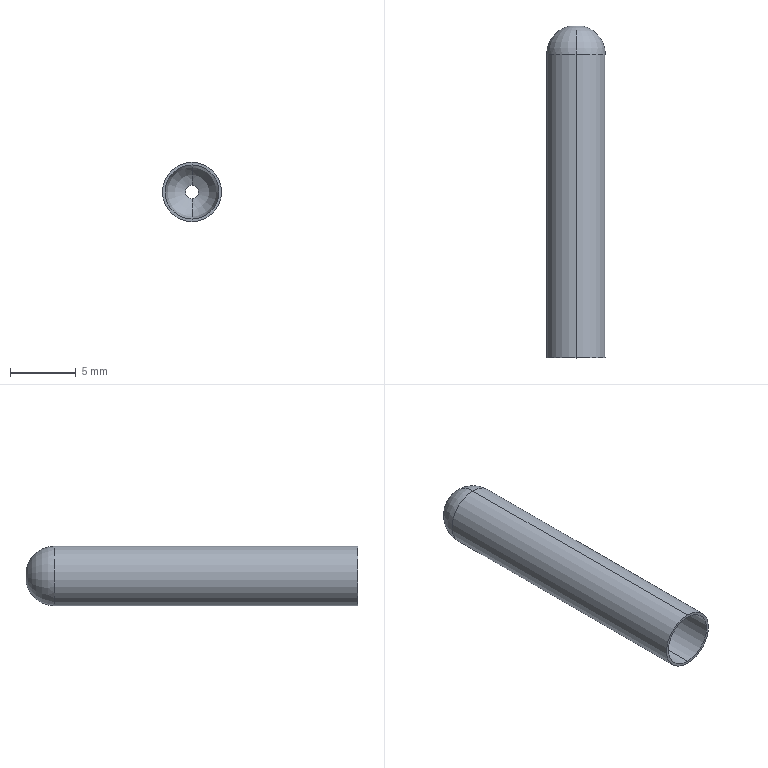Part | SolidWorks | features Revolution 1 | 1 solid | 11 faces | box 4.5 x 25.2 x 4.5 mm | volume 67.862 mm3 | cylinder 6 | torus 4 | plane 1 | commonest cylinder face diameters 1 x2 4.1 x2 4.5 x2
STEP:
#1=CARTESIAN_POINT('',(0.,23.047,2.05));
#2=VERTEX_POINT('',#1);
#3=CARTESIAN_POINT('',(0.,23.047,-2.05));
#4=VERTEX_POINT('',#3);
#5=CARTESIAN_POINT('',(0.,23.047,0.));
#6=DIRECTION('',(0.,-1.,0.));
#7=DIRECTION('',(0.,0.,-1.));
#8=AXIS2_PLACEMENT_3D('',#5,#6,#7);
#9=CIRCLE('',#8,2.05);
#10=EDGE_CURVE('',#2,#4,#9,.T.);
#11=ORIENTED_EDGE('',*,*,#10,.F.);
#12=CARTESIAN_POINT('',(0.,0.,2.05));
#13=VERTEX_POINT('',#12);
#14=CARTESIAN_POINT('',(0.,0.,2.05));
#15=DIRECTION('',(0.,-1.,0.));
#16=VECTOR('',#15,1000.);
#17=LINE('',#14,#16);
#18=EDGE_CURVE('',#2,#13,#17,.T.);
#19=ORIENTED_EDGE('',*,*,#18,.T.);
#20=CARTESIAN_POINT('',(0.,0.,-2.05));
#21=VERTEX_POINT('',#20);
#22=CARTESIAN_POINT('',(0.,0.,0.));
#23=DIRECTION('',(0.,-1.,0.));
#24=DIRECTION('',(0.,0.,-1.));
#25=AXIS2_PLACEMENT_3D('',#22,#23,#24);
#26=CIRCLE('',#25,2.05);
#27=EDGE_CURVE('',#13,#21,#26,.T.);
#28=ORIENTED_EDGE('',*,*,#27,.T.);
#29=CARTESIAN_POINT('',(0.,0.,-2.05));
#30=DIRECTION('',(0.,-1.,0.));
#31=VECTOR('',#30,1000.);
#32=LINE('',#29,#31);
#33=EDGE_CURVE('',#4,#21,#32,.T.);
#34=ORIENTED_EDGE('',*,*,#33,.F.);
#35=EDGE_LOOP('',(#11,#19,#28,#34));
#36=FACE_OUTER_BOUND('',#35,.T.);
#37=CARTESIAN_POINT('',(0.,0.,0.));
#38=DIRECTION('',(0.,-1.,0.));
#39=DIRECTION('',(0.,0.,-1.));
#40=AXIS2_PLACEMENT_3D('',#37,#38,#39);
#41=CYLINDRICAL_SURFACE('',#40,2.05);
#42=ADVANCED_FACE('',(#36),#41,.F.);
#43=CARTESIAN_POINT('',(0.,24.995,0.5));
#44=VERTEX_POINT('',#43);
#45=CARTESIAN_POINT('',(0.,24.995,-0.5));
#46=VERTEX_POINT('',#45);
#47=CARTESIAN_POINT('',(0.,24.995,0.));
#48=DIRECTION('',(0.,-1.,0.));
#49=DIRECTION('',(0.,0.,-1.));
#50=AXIS2_PLACEMENT_3D('',#47,#48,#49);
#51=CIRCLE('',#50,0.5);
#52=EDGE_CURVE('',#44,#46,#51,.T.);
#53=ORIENTED_EDGE('',*,*,#52,.F.);
#54=CARTESIAN_POINT('',(0.,23.047,0.05));
#55=DIRECTION('',(1.,0.,0.));
#56=DIRECTION('',(0.,0.,-1.));
#57=AXIS2_PLACEMENT_3D('',#54,#55,#56);
#58=CIRCLE('',#57,2.);
#59=EDGE_CURVE('',#44,#2,#58,.T.);
#60=ORIENTED_EDGE('',*,*,#59,.T.);
#61=ORIENTED_EDGE('',*,*,#10,.T.);
#62=CARTESIAN_POINT('',(0.,23.047,-0.05));
#63=DIRECTION('',(-1.,0.,0.));
#64=DIRECTION('',(0.,0.,1.));
#65=AXIS2_PLACEMENT_3D('',#62,#63,#64);
#66=CIRCLE('',#65,2.);
#67=EDGE_CURVE('',#46,#4,#66,.T.);
#68=ORIENTED_EDGE('',*,*,#67,.F.);
#69=EDGE_LOOP('',(#53,#60,#61,#68));
#70=FACE_OUTER_BOUND('',#69,.T.);
#71=CARTESIAN_POINT('',(0.,23.047,0.));
#72=DIRECTION('',(0.,-1.,0.));
#73=DIRECTION('',(0.,0.,-1.));
#74=AXIS2_PLACEMENT_3D('',#71,#72,#73);
#75=TOROIDAL_SURFACE('',#74,0.05,2.);
#76=ADVANCED_FACE('',(#70),#75,.F.);
#77=CARTESIAN_POINT('',(0.,25.2,0.5));
#78=VERTEX_POINT('',#77);
#79=CARTESIAN_POINT('',(0.,25.2,-0.5));
#80=VERTEX_POINT('',#79);
#81=CARTESIAN_POINT('',(0.,25.2,0.));
#82=DIRECTION('',(0.,-1.,0.));
#83=DIRECTION('',(0.,0.,-1.));
#84=AXIS2_PLACEMENT_3D('',#81,#82,#83);
#85=CIRCLE('',#84,0.5);
#86=EDGE_CURVE('',#78,#80,#85,.T.);
#87=ORIENTED_EDGE('',*,*,#86,.F.);
#88=CARTESIAN_POINT('',(0.,0.,0.5));
#89=DIRECTION('',(0.,-1.,0.));
#90=VECTOR('',#89,1000.);
#91=LINE('',#88,#90);
#92=EDGE_CURVE('',#78,#44,#91,.T.);
#93=ORIENTED_EDGE('',*,*,#92,.T.);
#94=ORIENTED_EDGE('',*,*,#52,.T.);
#95=CARTESIAN_POINT('',(0.,0.,-0.5));
#96=DIRECTION('',(0.,-1.,0.));
#97=VECTOR('',#96,1000.);
#98=LINE('',#95,#97);
#99=EDGE_CURVE('',#80,#46,#98,.T.);
#100=ORIENTED_EDGE('',*,*,#99,.F.);
#101=EDGE_LOOP('',(#87,#93,#94,#100));
#102=FACE_OUTER_BOUND('',#101,.T.);
#103=CARTESIAN_POINT('',(0.,0.,0.));
#104=DIRECTION('',(0.,-1.,0.));
#105=DIRECTION('',(0.,0.,-1.));
#106=AXIS2_PLACEMENT_3D('',#103,#104,#105);
#107=CYLINDRICAL_SURFACE('',#106,0.5);
#108=ADVANCED_FACE('',(#102),#107,.F.);
#109=CARTESIAN_POINT('',(0.,25.2,0.));
#110=DIRECTION('',(0.,-1.,0.));
#111=DIRECTION('',(0.,0.,-1.));
#112=AXIS2_PLACEMENT_3D('',#109,#110,#111);
#113=CIRCLE('',#112,0.5);
#114=EDGE_CURVE('',#80,#78,#113,.T.);
#115=ORIENTED_EDGE('',*,*,#114,.T.);
#116=CARTESIAN_POINT('',(0.,23.047,2.25));
#117=VERTEX_POINT('',#116);
#118=CARTESIAN_POINT('',(0.,23.047,0.05));
#119=DIRECTION('',(1.,0.,0.));
#120=DIRECTION('',(0.,0.,-1.));
#121=AXIS2_PLACEMENT_3D('',#118,#119,#120);
#122=CIRCLE('',#121,2.2);
#123=EDGE_CURVE('',#78,#117,#122,.T.);
#124=ORIENTED_EDGE('',*,*,#123,.T.);
#125=CARTESIAN_POINT('',(0.,23.047,-2.25));
#126=VERTEX_POINT('',#125);
#127=CARTESIAN_POINT('',(0.,23.047,0.));
#128=DIRECTION('',(0.,-1.,0.));
#129=DIRECTION('',(0.,0.,-1.));
#130=AXIS2_PLACEMENT_3D('',#127,#128,#129);
#131=CIRCLE('',#130,2.25);
#132=EDGE_CURVE('',#126,#117,#131,.T.);
#133=ORIENTED_EDGE('',*,*,#132,.F.);
#134=CARTESIAN_POINT('',(0.,23.047,-0.05));
#135=DIRECTION('',(-1.,0.,0.));
#136=DIRECTION('',(0.,0.,1.));
#137=AXIS2_PLACEMENT_3D('',#134,#135,#136);
#138=CIRCLE('',#137,2.2);
#139=EDGE_CURVE('',#80,#126,#138,.T.);
#140=ORIENTED_EDGE('',*,*,#139,.F.);
#141=EDGE_LOOP('',(#115,#124,#133,#140));
#142=FACE_OUTER_BOUND('',#141,.T.);
#143=CARTESIAN_POINT('',(0.,23.047,0.));
#144=DIRECTION('',(0.,-1.,0.));
#145=DIRECTION('',(0.,0.,-1.));
#146=AXIS2_PLACEMENT_3D('',#143,#144,#145);
#147=TOROIDAL_SURFACE('',#146,0.05,2.2);
#148=ADVANCED_FACE('',(#142),#147,.T.);
#149=ORIENTED_EDGE('',*,*,#132,.T.);
#150=CARTESIAN_POINT('',(0.,0.,2.25));
#151=VERTEX_POINT('',#150);
#152=CARTESIAN_POINT('',(0.,0.,2.25));
#153=DIRECTION('',(0.,-1.,0.));
#154=VECTOR('',#153,1000.);
#155=LINE('',#152,#154);
#156=EDGE_CURVE('',#117,#151,#155,.T.);
#157=ORIENTED_EDGE('',*,*,#156,.T.);
#158=CARTESIAN_POINT('',(0.,0.,-2.25));
#159=VERTEX_POINT('',#158);
#160=CARTESIAN_POINT('',(0.,0.,0.));
#161=DIRECTION('',(0.,-1.,0.));
#162=DIRECTION('',(0.,0.,-1.));
#163=AXIS2_PLACEMENT_3D('',#160,#161,#162);
#164=CIRCLE('',#163,2.25);
#165=EDGE_CURVE('',#159,#151,#164,.T.);
#166=ORIENTED_EDGE('',*,*,#165,.F.);
#167=CARTESIAN_POINT('',(0.,0.,-2.25));
#168=DIRECTION('',(0.,-1.,0.));
#169=VECTOR('',#168,1000.);
#170=LINE('',#167,#169);
#171=EDGE_CURVE('',#126,#159,#170,.T.);
#172=ORIENTED_EDGE('',*,*,#171,.F.);
#173=EDGE_LOOP('',(#149,#157,#166,#172));
#174=FACE_OUTER_BOUND('',#173,.T.);
#175=CARTESIAN_POINT('',(0.,0.,0.));
#176=DIRECTION('',(0.,-1.,0.));
#177=DIRECTION('',(0.,0.,-1.));
#178=AXIS2_PLACEMENT_3D('',#175,#176,#177);
#179=CYLINDRICAL_SURFACE('',#178,2.25);
#180=ADVANCED_FACE('',(#174),#179,.T.);
#181=CARTESIAN_POINT('',(0.,0.,0.));
#182=DIRECTION('',(0.,-1.,0.));
#183=DIRECTION('',(0.,0.,-1.));
#184=AXIS2_PLACEMENT_3D('',#181,#182,#183);
#185=CIRCLE('',#184,2.05);
#186=EDGE_CURVE('',#21,#13,#185,.T.);
#187=ORIENTED_EDGE('',*,*,#186,.F.);
#188=ORIENTED_EDGE('',*,*,#27,.F.);
#189=EDGE_LOOP('',(#187,#188));
#190=FACE_BOUND('',#189,.T.);
#191=ORIENTED_EDGE('',*,*,#165,.T.);
#192=CARTESIAN_POINT('',(0.,0.,0.));
#193=DIRECTION('',(0.,-1.,0.));
#194=DIRECTION('',(0.,0.,-1.));
#195=AXIS2_PLACEMENT_3D('',#192,#193,#194);
#196=CIRCLE('',#195,2.25);
#197=EDGE_CURVE('',#151,#159,#196,.T.);
#198=ORIENTED_EDGE('',*,*,#197,.T.);
#199=EDGE_LOOP('',(#191,#198));
#200=FACE_OUTER_BOUND('',#199,.T.);
#201=CARTESIAN_POINT('',(-2.25,0.,0.));
#202=DIRECTION('',(0.,1.,0.));
#203=DIRECTION('',(0.,0.,1.));
#204=AXIS2_PLACEMENT_3D('',#201,#202,#203);
#205=PLANE('',#204);
#206=ADVANCED_FACE('',(#190,#200),#205,.F.);
#207=ORIENTED_EDGE('',*,*,#156,.F.);
#208=CARTESIAN_POINT('',(0.,23.047,0.));
#209=DIRECTION('',(0.,-1.,0.));
#210=DIRECTION('',(0.,0.,-1.));
#211=AXIS2_PLACEMENT_3D('',#208,#209,#210);
#212=CIRCLE('',#211,2.25);
#213=EDGE_CURVE('',#117,#126,#212,.T.);
#214=ORIENTED_EDGE('',*,*,#213,.T.);
#215=ORIENTED_EDGE('',*,*,#171,.T.);
#216=ORIENTED_EDGE('',*,*,#197,.F.);
#217=EDGE_LOOP('',(#207,#214,#215,#216));
#218=FACE_OUTER_BOUND('',#217,.T.);
#219=CARTESIAN_POINT('',(0.,0.,0.));
#220=DIRECTION('',(0.,-1.,0.));
#221=DIRECTION('',(0.,0.,-1.));
#222=AXIS2_PLACEMENT_3D('',#219,#220,#221);
#223=CYLINDRICAL_SURFACE('',#222,2.25);
#224=ADVANCED_FACE('',(#218),#223,.T.);
#225=ORIENTED_EDGE('',*,*,#123,.F.);
#226=ORIENTED_EDGE('',*,*,#86,.T.);
#227=ORIENTED_EDGE('',*,*,#139,.T.);
#228=ORIENTED_EDGE('',*,*,#213,.F.);
#229=EDGE_LOOP('',(#225,#226,#227,#228));
#230=FACE_OUTER_BOUND('',#229,.T.);
#231=CARTESIAN_POINT('',(0.,23.047,0.));
#232=DIRECTION('',(0.,-1.,0.));
#233=DIRECTION('',(0.,0.,-1.));
#234=AXIS2_PLACEMENT_3D('',#231,#232,#233);
#235=TOROIDAL_SURFACE('',#234,0.05,2.2);
#236=ADVANCED_FACE('',(#230),#235,.T.);
#237=ORIENTED_EDGE('',*,*,#92,.F.);
#238=ORIENTED_EDGE('',*,*,#114,.F.);
#239=ORIENTED_EDGE('',*,*,#99,.T.);
#240=CARTESIAN_POINT('',(0.,24.995,0.));
#241=DIRECTION('',(0.,-1.,0.));
#242=DIRECTION('',(0.,0.,-1.));
#243=AXIS2_PLACEMENT_3D('',#240,#241,#242);
#244=CIRCLE('',#243,0.5);
#245=EDGE_CURVE('',#46,#44,#244,.T.);
#246=ORIENTED_EDGE('',*,*,#245,.T.);
#247=EDGE_LOOP('',(#237,#238,#239,#246));
#248=FACE_OUTER_BOUND('',#247,.T.);
#249=CARTESIAN_POINT('',(0.,0.,0.));
#250=DIRECTION('',(0.,-1.,0.));
#251=DIRECTION('',(0.,0.,-1.));
#252=AXIS2_PLACEMENT_3D('',#249,#250,#251);
#253=CYLINDRICAL_SURFACE('',#252,0.5);
#254=ADVANCED_FACE('',(#248),#253,.F.);
#255=ORIENTED_EDGE('',*,*,#59,.F.);
#256=ORIENTED_EDGE('',*,*,#245,.F.);
#257=ORIENTED_EDGE('',*,*,#67,.T.);
#258=CARTESIAN_POINT('',(0.,23.047,0.));
#259=DIRECTION('',(0.,-1.,0.));
#260=DIRECTION('',(0.,0.,-1.));
#261=AXIS2_PLACEMENT_3D('',#258,#259,#260);
#262=CIRCLE('',#261,2.05);
#263=EDGE_CURVE('',#4,#2,#262,.T.);
#264=ORIENTED_EDGE('',*,*,#263,.T.);
#265=EDGE_LOOP('',(#255,#256,#257,#264));
#266=FACE_OUTER_BOUND('',#265,.T.);
#267=CARTESIAN_POINT('',(0.,23.047,0.));
#268=DIRECTION('',(0.,-1.,0.));
#269=DIRECTION('',(0.,0.,-1.));
#270=AXIS2_PLACEMENT_3D('',#267,#268,#269);
#271=TOROIDAL_SURFACE('',#270,0.05,2.);
#272=ADVANCED_FACE('',(#266),#271,.F.);
#273=ORIENTED_EDGE('',*,*,#18,.F.);
#274=ORIENTED_EDGE('',*,*,#263,.F.);
#275=ORIENTED_EDGE('',*,*,#33,.T.);
#276=ORIENTED_EDGE('',*,*,#186,.T.);
#277=EDGE_LOOP('',(#273,#274,#275,#276));
#278=FACE_OUTER_BOUND('',#277,.T.);
#279=CARTESIAN_POINT('',(0.,0.,0.));
#280=DIRECTION('',(0.,-1.,0.));
#281=DIRECTION('',(0.,0.,-1.));
#282=AXIS2_PLACEMENT_3D('',#279,#280,#281);
#283=CYLINDRICAL_SURFACE('',#282,2.05);
#284=ADVANCED_FACE('',(#278),#283,.F.);
#285=CLOSED_SHELL('',(#42,#76,#108,#148,#180,#206,#224,#236,#254,#272,#284));
#286=MANIFOLD_SOLID_BREP('',#285);
#287=CARTESIAN_POINT('',(0.,0.,0.));
#288=DIRECTION('',(0.,0.,1.));
#289=DIRECTION('',(1.,0.,0.));
#290=AXIS2_PLACEMENT_3D('',#287,#288,#289);
#291=(LENGTH_UNIT()NAMED_UNIT(*)SI_UNIT(.MILLI.,.METRE.));
#292=UNCERTAINTY_MEASURE_WITH_UNIT(LENGTH_MEASURE(0.00001),#291,'','');
#293=(NAMED_UNIT(*)PLANE_ANGLE_UNIT()SI_UNIT($,.RADIAN.));
#294=(NAMED_UNIT(*)SI_UNIT($,.STERADIAN.)SOLID_ANGLE_UNIT());
#295=(GEOMETRIC_REPRESENTATION_CONTEXT(3)GLOBAL_UNCERTAINTY_ASSIGNED_CONTEXT((#292))GLOBAL_UNIT_ASSIGNED_CONTEXT((#291,#293,#294))REPRESENTATION_CONTEXT('',''));
#296=ADVANCED_BREP_SHAPE_REPRESENTATION('',(#286,#290),#295);